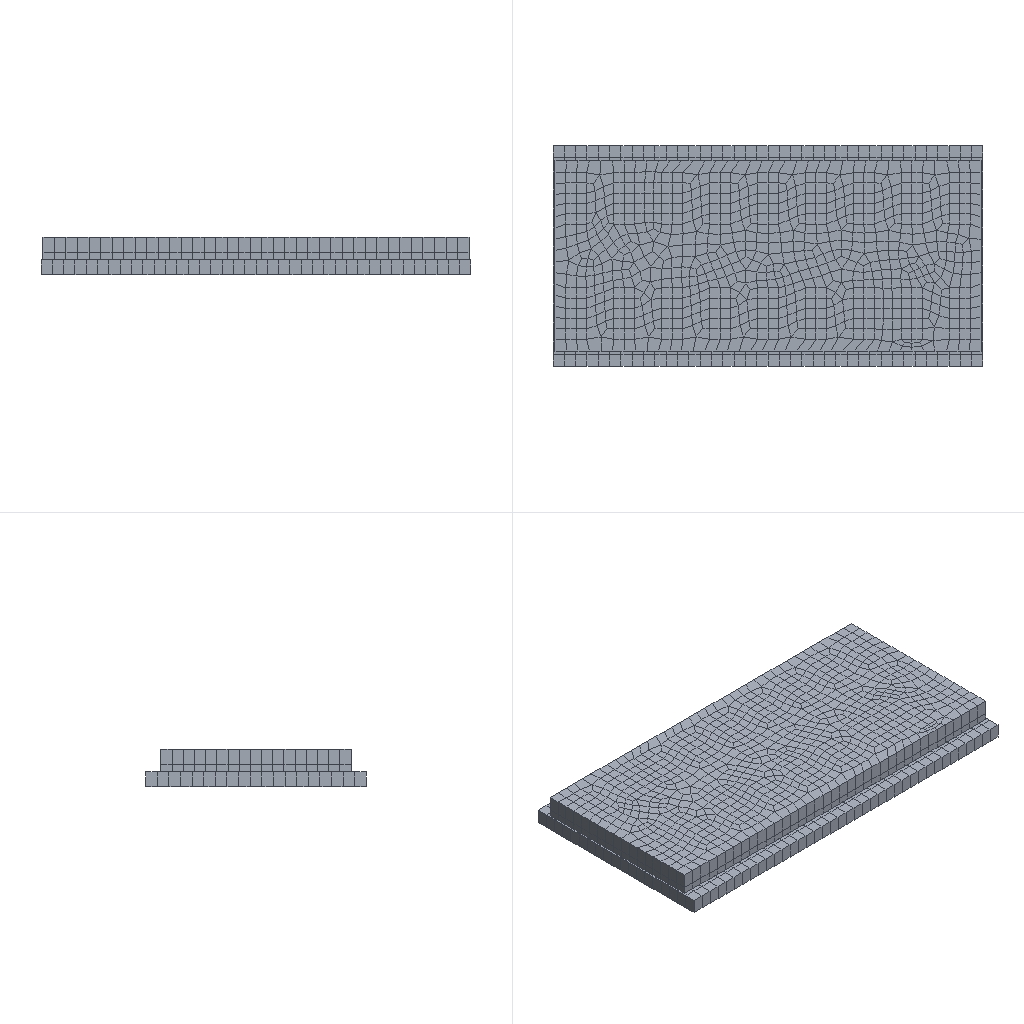Simulation study | abaqus
Set-up summary:
category,name,step,type,value,unit,region
solver,abaqus
solver,version,,,Abaqus/Standard 2020
units,not stated in the deck,,not stated
analysis,deck,,static,static
load_step,Step-1,Step-1,static
load_step,requested,,,1
mesh,nodes,,,5088
mesh,elements,,,2556
element_type,T3D2,,truss,400
element_type,C3D8R,,solid,2156
load,load commands in deck,,count,2
bc,support commands in deck,,count,1
material,DIZUOANDCHONGTIAN,,in results
material,GUIDAO,,in results
material,STEEL,,in results
check,setup vs results,,match,"per instance, exact: element labels, types and connectivity; labels of the nodes the elements use; coordinates of those nodes at SINGLE_PRECISION in 43 of 43 instance(s)"
Abaqus input file, long lists of numbers shortened:
*Heading
** Job name: Job-1 Model name: Model-1
** Generated by: Abaqus/CAE 2020
*Preprint, echo=NO, model=NO, history=NO, contact=NO
**
** PARTS
**
*Part, name=chongtian
*Node
      1,           0.,       -2500.,          94.
      2,           0.,  -2352.941,          94.
** (1366 more lines like these left out)
*Element, type=C3D8R
  1,   37,   38,   56,   55,    1,    2,   20,   19
  2,   38,   39,   57,   56,    2,    3,   21,   20
** (627 more lines like these left out)
*Nset, nset=Set-1, generate
    1,  1368,     1
*Elset, elset=Set-1, generate
   1,  629,    1
** Section: chongtian
*Solid Section, elset=Set-1, material=dizuoandchongtian
,
*End Part
**
*Part, name=dizuo
*Node
      1,           0.,       -2900.,         196.
      2,           0.,  -2747.368,         196.
** (1558 more lines like these left out)
*Element, type=C3D8R
  1,   41,   42,   62,   61,    1,    2,   22,   21
  2,   42,   43,   63,   62,    2,    3,   23,   22
** (720 more lines like these left out)
*Nset, nset=Set-1, generate
    1,  1560,     1
*Elset, elset=Set-1, generate
   1,  722,    1
** Section: chongtian
*Solid Section, elset=Set-1, material=dizuoandchongtian
,
*End Part
**
*Part, name=guidao
*Node
      1,       5182.5,       -1669.,         200.
      2,       5182.5,       -2344.,         200.
** (1718 more lines like these left out)
*Element, type=C3D8R
  1,   86,  361,   77,    1,  946, 1221,  937,  861
  2,  361,  362,   78,   77, 1221, 1222,  938,  937
** (803 more lines like these left out)
*Nset, nset=Set-1, generate
    1,  1720,     1
*Elset, elset=Set-1, generate
   1,  805,    1
** Section: guidao
*Solid Section, elset=Set-1, material=guidao
,
*End Part
**
*Part, name=heng-jin
*Node
      1,           0.,           0.,           0.
      2,           0.,       -243.5,           0.
** (9 more lines like these left out)
*Element, type=T3D2
 1,  1,  2
 2,  2,  3
** (8 more lines like these left out)
*Nset, nset=Set-2, generate
  1,  11,   1
*Elset, elset=Set-2, generate
  1,  10,   1
** Section: steel
*Solid Section, elset=Set-2, material=steel
78.5,
*End Part
**
*Part, name=zong-jin
*Node
      1,           0.,           0.,           0.
      2,           0.,        -552.,           0.
** (9 more lines like these left out)
*Element, type=T3D2
 1,  1,  2
 2,  2,  3
** (8 more lines like these left out)
*Nset, nset=Set-2, generate
  1,  11,   1
*Elset, elset=Set-2, generate
  1,  10,   1
** Section: steel
*Solid Section, elset=Set-2, material=steel
78.5,
*End Part
**
**
** ASSEMBLY
**
*Assembly, name=Assembly
**
*Instance, name=chongtian-1, part=chongtian
         25.,        -200.,         196.
*End Instance
**
*Instance, name=dizuo-1, part=dizuo
*End Instance
**
*Instance, name=guidao-1, part=guidao
         25.,        -200.,         290.
*End Instance
**
*Instance, name=heng-jin-1, part=heng-jin
        175.,       -232.5,         390.
*End Instance
**
*Instance, name=zong-jin-1, part=zong-jin
         75.,       -232.5,         350.
         75.,       -232.5,         350.,          75.,       -232.5, 351., 90.
*End Instance
**
*Instance, name=zong-jin-1-lin-1-2-1, part=zong-jin
         75.,       -572.5,         350.
         75.,       -572.5,         350.,          75.,       -572.5, 351., 90.
*End Instance
**
*Instance, name=zong-jin-1-lin-1-3, part=zong-jin
         75.,       -912.5,         350.
         75.,       -912.5,         350.,          75.,       -912.5, 351., 90.
*End Instance
**
*Instance, name=zong-jin-1-lin-1-4, part=zong-jin
         75.,      -1252.5,         350.
         75.,      -1252.5,         350.,          75.,      -1252.5, 351., 90.
*End Instance
**
*Instance, name=zong-jin-1-lin-1-5, part=zong-jin
         75.,      -1592.5,         350.
         75.,      -1592.5,         350.,          75.,      -1592.5, 351., 90.
*End Instance
**
*Instance, name=zong-jin-1-lin-1-6, part=zong-jin
         75.,      -1932.5,         350.
         75.,      -1932.5,         350.,          75.,      -1932.5, 351., 90.
*End Instance
**
*Instance, name=zong-jin-1-lin-1-7, part=zong-jin
         75.,      -2272.5,         350.
         75.,      -2272.5,         350.,          75.,      -2272.5, 351., 90.
*End Instance
**
*Instance, name=zong-jin-1-lin-1-8, part=zong-jin
         75.,      -2612.5,         350.
         75.,      -2612.5,         350.,          75.,      -2612.5, 351., 90.
*End Instance
**
*Instance, name=zong-jin-1-lin-2-1-1, part=zong-jin
         75.,       -232.5,         430.
         75.,       -232.5,         430.,          75.,       -232.5, 431., 90.
*End Instance
**
*Instance, name=zong-jin-1-lin-2-2-1, part=zong-jin
         75.,       -572.5,         430.
         75.,       -572.5,         430.,          75.,       -572.5, 431., 90.
*End Instance
**
*Instance, name=zong-jin-1-lin-2-3, part=zong-jin
         75.,       -912.5,         430.
         75.,       -912.5,         430.,          75.,       -912.5, 431., 90.
*End Instance
**
*Instance, name=zong-jin-1-lin-2-4, part=zong-jin
         75.,      -1252.5,         430.
         75.,      -1252.5,         430.,          75.,      -1252.5, 431., 90.
*End Instance
**
*Instance, name=zong-jin-1-lin-2-5, part=zong-jin
         75.,      -1592.5,         430.
         75.,      -1592.5,         430.,          75.,      -1592.5, 431., 90.
*End Instance
**
*Instance, name=zong-jin-1-lin-2-6, part=zong-jin
         75.,      -1932.5,         430.
         75.,      -1932.5,         430.,          75.,      -1932.5, 431., 90.
*End Instance
**
*Instance, name=zong-jin-1-lin-2-7, part=zong-jin
         75.,      -2272.5,         430.
         75.,      -2272.5,         430.,          75.,      -2272.5, 431., 90.
*End Instance
**
*Instance, name=zong-jin-1-lin-2-8, part=zong-jin
         75.,      -2612.5,         430.
         75.,      -2612.5,         430.,          75.,      -2612.5, 431., 90.
*End Instance
**
*Instance, name=heng-jin-1-lin-2-1-1, part=heng-jin
        405.,       -232.5,         390.
*End Instance
**
*Instance, name=heng-jin-1-lin-3-1-1, part=heng-jin
        635.,       -232.5,         390.
*End Instance
**
*Instance, name=heng-jin-1-lin-4-1-1, part=heng-jin
        865.,       -232.5,         390.
*End Instance
**
*Instance, name=heng-jin-1-lin-5-1-1, part=heng-jin
       1095.,       -232.5,         390.
*End Instance
**
*Instance, name=heng-jin-1-lin-6-1-1, part=heng-jin
       1325.,       -232.5,         390.
*End Instance
**
*Instance, name=heng-jin-1-lin-7-1-1, part=heng-jin
       1555.,       -232.5,         390.
*End Instance
**
*Instance, name=heng-jin-1-lin-8-1-1, part=heng-jin
       1785.,       -232.5,         390.
*End Instance
**
*Instance, name=heng-jin-1-lin-9-1, part=heng-jin
       2015.,       -232.5,         390.
*End Instance
**
*Instance, name=heng-jin-1-lin-10-1, part=heng-jin
       2245.,       -232.5,         390.
*End Instance
**
*Instance, name=heng-jin-1-lin-11-1, part=heng-jin
       2475.,       -232.5,         390.
*End Instance
**
*Instance, name=heng-jin-1-lin-12-1, part=heng-jin
       2705.,       -232.5,         390.
*End Instance
**
*Instance, name=heng-jin-1-lin-13-1, part=heng-jin
       2935.,       -232.5,         390.
*End Instance
**
*Instance, name=heng-jin-1-lin-14-1, part=heng-jin
       3165.,       -232.5,         390.
*End Instance
**
*Instance, name=heng-jin-1-lin-15-1, part=heng-jin
       3395.,       -232.5,         390.
*End Instance
**
*Instance, name=heng-jin-1-lin-16-1, part=heng-jin
       3625.,       -232.5,         390.
*End Instance
**
*Instance, name=heng-jin-1-lin-17-1, part=heng-jin
       3855.,       -232.5,         390.
*End Instance
**
*Instance, name=heng-jin-1-lin-18-1, part=heng-jin
       4085.,       -232.5,         390.
*End Instance
**
*Instance, name=heng-jin-1-lin-19-1, part=heng-jin
       4315.,       -232.5,         390.
*End Instance
**
*Instance, name=heng-jin-1-lin-20-1, part=heng-jin
       4545.,       -232.5,         390.
*End Instance
**
*Instance, name=heng-jin-1-lin-21-1, part=heng-jin
       4775.,       -232.5,         390.
*End Instance
**
*Instance, name=heng-jin-1-lin-22-1, part=heng-jin
       5005.,       -232.5,         390.
*End Instance
**
*Instance, name=heng-jin-1-lin-23-1, part=heng-jin
       5235.,       -232.5,         390.
*End Instance
**
*Instance, name=heng-jin-1-lin-24-1, part=heng-jin
       5465.,       -232.5,         390.
*End Instance
**
*Nset, nset=Set-3, instance=heng-jin-1, generate
  1,  11,   1
*Nset, nset=Set-3, instance=zong-jin-1, generate
  1,  11,   1
*Elset, elset=Set-3, instance=heng-jin-1, generate
  1,  10,   1
*Elset, elset=Set-3, instance=zong-jin-1, generate
  1,  10,   1
*Nset, nset=Set-4, instance=dizuo-1
   21,   22,   23,   24,   25,   26,   27,   28,   29,   30,   31,   32,   33,   34,   35,   36
   37,   38,   39,   40,   61,   62,   63,   64,   65,   66,   67,   68,   69,   70,   71,   72
** (47 more lines like these left out)
*Elset, elset=Set-4, instance=dizuo-1, generate
   1,  722,    1
*Nset, nset=Set-7, instance=heng-jin-1, generate
  1,  11,   1
*Nset, nset=Set-7, instance=zong-jin-1, generate
  1,  11,   1
*Nset, nset=Set-7, instance=zong-jin-1-lin-1-2-1, generate
  1,  11,   1
*Nset, nset=Set-7, instance=zong-jin-1-lin-1-4, generate
  1,  11,   1
*Nset, nset=Set-7, instance=zong-jin-1-lin-1-6, generate
  1,  11,   1
*Nset, nset=Set-7, instance=zong-jin-1-lin-2-6, generate
  1,  11,   1
*Nset, nset=Set-7, instance=heng-jin-1-lin-7-1-1, generate
  1,  11,   1
*Nset, nset=Set-7, instance=heng-jin-1-lin-23-1, generate
  1,  11,   1
*Nset, nset=Set-7, instance=heng-jin-1-lin-15-1, generate
  1,  11,   1
*Nset, nset=Set-7, instance=zong-jin-1-lin-2-2-1, generate
  1,  11,   1
*Nset, nset=Set-7, instance=heng-jin-1-lin-11-1, generate
  1,  11,   1
*Nset, nset=Set-7, instance=heng-jin-1-lin-3-1-1, generate
  1,  11,   1
*Nset, nset=Set-7, instance=heng-jin-1-lin-19-1, generate
  1,  11,   1
*Nset, nset=Set-7, instance=zong-jin-1-lin-1-8, generate
  1,  11,   1
*Nset, nset=Set-7, instance=zong-jin-1-lin-2-8, generate
  1,  11,   1
*Nset, nset=Set-7, instance=heng-jin-1-lin-9-1, generate
  1,  11,   1
*Nset, nset=Set-7, instance=heng-jin-1-lin-17-1, generate
  1,  11,   1
*Nset, nset=Set-7, instance=zong-jin-1-lin-2-4, generate
  1,  11,   1
*Nset, nset=Set-7, instance=heng-jin-1-lin-13-1, generate
  1,  11,   1
*Nset, nset=Set-7, instance=heng-jin-1-lin-5-1-1, generate
  1,  11,   1
*Nset, nset=Set-7, instance=heng-jin-1-lin-21-1, generate
  1,  11,   1
*Nset, nset=Set-7, instance=zong-jin-1-lin-1-3, generate
  1,  11,   1
*Nset, nset=Set-7, instance=zong-jin-1-lin-1-7, generate
  1,  11,   1
*Nset, nset=Set-7, instance=zong-jin-1-lin-2-7, generate
  1,  11,   1
*Nset, nset=Set-7, instance=heng-jin-1-lin-8-1-1, generate
  1,  11,   1
*Nset, nset=Set-7, instance=heng-jin-1-lin-24-1, generate
  1,  11,   1
*Nset, nset=Set-7, instance=heng-jin-1-lin-16-1, generate
  1,  11,   1
*Nset, nset=Set-7, instance=zong-jin-1-lin-2-3, generate
  1,  11,   1
*Nset, nset=Set-7, instance=heng-jin-1-lin-12-1, generate
  1,  11,   1
*Nset, nset=Set-7, instance=heng-jin-1-lin-4-1-1, generate
  1,  11,   1
*Nset, nset=Set-7, instance=heng-jin-1-lin-20-1, generate
  1,  11,   1
*Nset, nset=Set-7, instance=zong-jin-1-lin-1-5, generate
  1,  11,   1
*Nset, nset=Set-7, instance=zong-jin-1-lin-2-1-1, generate
  1,  11,   1
*Nset, nset=Set-7, instance=heng-jin-1-lin-10-1, generate
  1,  11,   1
*Nset, nset=Set-7, instance=heng-jin-1-lin-2-1-1, generate
  1,  11,   1
*Nset, nset=Set-7, instance=heng-jin-1-lin-18-1, generate
  1,  11,   1
*Nset, nset=Set-7, instance=zong-jin-1-lin-2-5, generate
  1,  11,   1
*Nset, nset=Set-7, instance=heng-jin-1-lin-14-1, generate
  1,  11,   1
*Nset, nset=Set-7, instance=heng-jin-1-lin-6-1-1, generate
  1,  11,   1
*Nset, nset=Set-7, instance=heng-jin-1-lin-22-1, generate
  1,  11,   1
*Elset, elset=Set-7, instance=heng-jin-1, generate
  1,  10,   1
*Elset, elset=Set-7, instance=zong-jin-1, generate
  1,  10,   1
*Elset, elset=Set-7, instance=zong-jin-1-lin-1-2-1, generate
  1,  10,   1
*Elset, elset=Set-7, instance=zong-jin-1-lin-1-4, generate
  1,  10,   1
*Elset, elset=Set-7, instance=zong-jin-1-lin-1-6, generate
  1,  10,   1
*Elset, elset=Set-7, instance=zong-jin-1-lin-2-6, generate
  1,  10,   1
*Elset, elset=Set-7, instance=heng-jin-1-lin-7-1-1, generate
  1,  10,   1
*Elset, elset=Set-7, instance=heng-jin-1-lin-23-1, generate
  1,  10,   1
*Elset, elset=Set-7, instance=heng-jin-1-lin-15-1, generate
  1,  10,   1
*Elset, elset=Set-7, instance=zong-jin-1-lin-2-2-1, generate
  1,  10,   1
*Elset, elset=Set-7, instance=heng-jin-1-lin-11-1, generate
  1,  10,   1
*Elset, elset=Set-7, instance=heng-jin-1-lin-3-1-1, generate
  1,  10,   1
*Elset, elset=Set-7, instance=heng-jin-1-lin-19-1, generate
  1,  10,   1
*Elset, elset=Set-7, instance=zong-jin-1-lin-1-8, generate
  1,  10,   1
*Elset, elset=Set-7, instance=zong-jin-1-lin-2-8, generate
  1,  10,   1
*Elset, elset=Set-7, instance=heng-jin-1-lin-9-1, generate
  1,  10,   1
*Elset, elset=Set-7, instance=heng-jin-1-lin-17-1, generate
  1,  10,   1
*Elset, elset=Set-7, instance=zong-jin-1-lin-2-4, generate
  1,  10,   1
*Elset, elset=Set-7, instance=heng-jin-1-lin-13-1, generate
  1,  10,   1
*Elset, elset=Set-7, instance=heng-jin-1-lin-5-1-1, generate
  1,  10,   1
*Elset, elset=Set-7, instance=heng-jin-1-lin-21-1, generate
  1,  10,   1
*Elset, elset=Set-7, instance=zong-jin-1-lin-1-3, generate
  1,  10,   1
*Elset, elset=Set-7, instance=zong-jin-1-lin-1-7, generate
  1,  10,   1
*Elset, elset=Set-7, instance=zong-jin-1-lin-2-7, generate
  1,  10,   1
*Elset, elset=Set-7, instance=heng-jin-1-lin-8-1-1, generate
  1,  10,   1
*Elset, elset=Set-7, instance=heng-jin-1-lin-24-1, generate
  1,  10,   1
*Elset, elset=Set-7, instance=heng-jin-1-lin-16-1, generate
  1,  10,   1
*Elset, elset=Set-7, instance=zong-jin-1-lin-2-3, generate
  1,  10,   1
*Elset, elset=Set-7, instance=heng-jin-1-lin-12-1, generate
  1,  10,   1
*Elset, elset=Set-7, instance=heng-jin-1-lin-4-1-1, generate
  1,  10,   1
*Elset, elset=Set-7, instance=heng-jin-1-lin-20-1, generate
  1,  10,   1
*Elset, elset=Set-7, instance=zong-jin-1-lin-1-5, generate
  1,  10,   1
*Elset, elset=Set-7, instance=zong-jin-1-lin-2-1-1, generate
  1,  10,   1
*Elset, elset=Set-7, instance=heng-jin-1-lin-10-1, generate
  1,  10,   1
*Elset, elset=Set-7, instance=heng-jin-1-lin-2-1-1, generate
  1,  10,   1
*Elset, elset=Set-7, instance=heng-jin-1-lin-18-1, generate
  1,  10,   1
*Elset, elset=Set-7, instance=zong-jin-1-lin-2-5, generate
  1,  10,   1
*Elset, elset=Set-7, instance=heng-jin-1-lin-14-1, generate
  1,  10,   1
*Elset, elset=Set-7, instance=heng-jin-1-lin-6-1-1, generate
  1,  10,   1
*Elset, elset=Set-7, instance=heng-jin-1-lin-22-1, generate
  1,  10,   1
*Nset, nset=m_Set-1, instance=heng-jin-1, generate
  1,  11,   1
*Nset, nset=m_Set-1, instance=zong-jin-1, generate
  1,  11,   1
*Elset, elset=m_Set-1, instance=heng-jin-1, generate
  1,  10,   1
*Elset, elset=m_Set-1, instance=zong-jin-1, generate
  1,  10,   1
*Nset, nset=m_Set-5, instance=heng-jin-1, generate
  1,  11,   1
*Nset, nset=m_Set-5, instance=zong-jin-1, generate
  1,  11,   1
*Nset, nset=m_Set-5, instance=zong-jin-1-lin-1-2-1, generate
  1,  11,   1
*Nset, nset=m_Set-5, instance=zong-jin-1-lin-1-4, generate
  1,  11,   1
*Nset, nset=m_Set-5, instance=zong-jin-1-lin-1-6, generate
  1,  11,   1
*Nset, nset=m_Set-5, instance=zong-jin-1-lin-2-6, generate
  1,  11,   1
*Nset, nset=m_Set-5, instance=heng-jin-1-lin-7-1-1, generate
  1,  11,   1
*Nset, nset=m_Set-5, instance=heng-jin-1-lin-23-1, generate
  1,  11,   1
*Nset, nset=m_Set-5, instance=heng-jin-1-lin-15-1, generate
  1,  11,   1
*Nset, nset=m_Set-5, instance=zong-jin-1-lin-2-2-1, generate
  1,  11,   1
*Nset, nset=m_Set-5, instance=heng-jin-1-lin-11-1, generate
  1,  11,   1
*Nset, nset=m_Set-5, instance=heng-jin-1-lin-3-1-1, generate
  1,  11,   1
*Nset, nset=m_Set-5, instance=heng-jin-1-lin-19-1, generate
  1,  11,   1
*Nset, nset=m_Set-5, instance=zong-jin-1-lin-1-8, generate
  1,  11,   1
*Nset, nset=m_Set-5, instance=zong-jin-1-lin-2-8, generate
  1,  11,   1
*Nset, nset=m_Set-5, instance=heng-jin-1-lin-9-1, generate
  1,  11,   1
*Nset, nset=m_Set-5, instance=heng-jin-1-lin-17-1, generate
  1,  11,   1
*Nset, nset=m_Set-5, instance=zong-jin-1-lin-2-4, generate
  1,  11,   1
*Nset, nset=m_Set-5, instance=heng-jin-1-lin-13-1, generate
  1,  11,   1
*Nset, nset=m_Set-5, instance=heng-jin-1-lin-5-1-1, generate
  1,  11,   1
*Nset, nset=m_Set-5, instance=heng-jin-1-lin-21-1, generate
  1,  11,   1
*Nset, nset=m_Set-5, instance=zong-jin-1-lin-1-3, generate
  1,  11,   1
*Nset, nset=m_Set-5, instance=zong-jin-1-lin-1-7, generate
  1,  11,   1
*Nset, nset=m_Set-5, instance=zong-jin-1-lin-2-7, generate
  1,  11,   1
*Nset, nset=m_Set-5, instance=heng-jin-1-lin-8-1-1, generate
  1,  11,   1
*Nset, nset=m_Set-5, instance=heng-jin-1-lin-24-1, generate
  1,  11,   1
*Nset, nset=m_Set-5, instance=heng-jin-1-lin-16-1, generate
  1,  11,   1
*Nset, nset=m_Set-5, instance=zong-jin-1-lin-2-3, generate
  1,  11,   1
*Nset, nset=m_Set-5, instance=heng-jin-1-lin-12-1, generate
  1,  11,   1
*Nset, nset=m_Set-5, instance=heng-jin-1-lin-4-1-1, generate
  1,  11,   1
*Nset, nset=m_Set-5, instance=heng-jin-1-lin-20-1, generate
  1,  11,   1
*Nset, nset=m_Set-5, instance=zong-jin-1-lin-1-5, generate
  1,  11,   1
*Nset, nset=m_Set-5, instance=zong-jin-1-lin-2-1-1, generate
  1,  11,   1
*Nset, nset=m_Set-5, instance=heng-jin-1-lin-10-1, generate
  1,  11,   1
*Nset, nset=m_Set-5, instance=heng-jin-1-lin-2-1-1, generate
  1,  11,   1
*Nset, nset=m_Set-5, instance=heng-jin-1-lin-18-1, generate
  1,  11,   1
*Nset, nset=m_Set-5, instance=zong-jin-1-lin-2-5, generate
  1,  11,   1
*Nset, nset=m_Set-5, instance=heng-jin-1-lin-14-1, generate
  1,  11,   1
*Nset, nset=m_Set-5, instance=heng-jin-1-lin-6-1-1, generate
  1,  11,   1
*Nset, nset=m_Set-5, instance=heng-jin-1-lin-22-1, generate
  1,  11,   1
*Elset, elset=m_Set-5, instance=heng-jin-1, generate
  1,  10,   1
*Elset, elset=m_Set-5, instance=zong-jin-1, generate
  1,  10,   1
*Elset, elset=m_Set-5, instance=zong-jin-1-lin-1-2-1, generate
  1,  10,   1
*Elset, elset=m_Set-5, instance=zong-jin-1-lin-1-4, generate
  1,  10,   1
*Elset, elset=m_Set-5, instance=zong-jin-1-lin-1-6, generate
  1,  10,   1
*Elset, elset=m_Set-5, instance=zong-jin-1-lin-2-6, generate
  1,  10,   1
*Elset, elset=m_Set-5, instance=heng-jin-1-lin-7-1-1, generate
  1,  10,   1
*Elset, elset=m_Set-5, instance=heng-jin-1-lin-23-1, generate
  1,  10,   1
*Elset, elset=m_Set-5, instance=heng-jin-1-lin-15-1, generate
  1,  10,   1
*Elset, elset=m_Set-5, instance=zong-jin-1-lin-2-2-1, generate
  1,  10,   1
*Elset, elset=m_Set-5, instance=heng-jin-1-lin-11-1, generate
  1,  10,   1
*Elset, elset=m_Set-5, instance=heng-jin-1-lin-3-1-1, generate
  1,  10,   1
*Elset, elset=m_Set-5, instance=heng-jin-1-lin-19-1, generate
  1,  10,   1
*Elset, elset=m_Set-5, instance=zong-jin-1-lin-1-8, generate
  1,  10,   1
*Elset, elset=m_Set-5, instance=zong-jin-1-lin-2-8, generate
  1,  10,   1
*Elset, elset=m_Set-5, instance=heng-jin-1-lin-9-1, generate
  1,  10,   1
*Elset, elset=m_Set-5, instance=heng-jin-1-lin-17-1, generate
  1,  10,   1
*Elset, elset=m_Set-5, instance=zong-jin-1-lin-2-4, generate
  1,  10,   1
*Elset, elset=m_Set-5, instance=heng-jin-1-lin-13-1, generate
  1,  10,   1
*Elset, elset=m_Set-5, instance=heng-jin-1-lin-5-1-1, generate
  1,  10,   1
*Elset, elset=m_Set-5, instance=heng-jin-1-lin-21-1, generate
  1,  10,   1
*Elset, elset=m_Set-5, instance=zong-jin-1-lin-1-3, generate
  1,  10,   1
*Elset, elset=m_Set-5, instance=zong-jin-1-lin-1-7, generate
  1,  10,   1
*Elset, elset=m_Set-5, instance=zong-jin-1-lin-2-7, generate
  1,  10,   1
*Elset, elset=m_Set-5, instance=heng-jin-1-lin-8-1-1, generate
  1,  10,   1
*Elset, elset=m_Set-5, instance=heng-jin-1-lin-24-1, generate
  1,  10,   1
*Elset, elset=m_Set-5, instance=heng-jin-1-lin-16-1, generate
  1,  10,   1
*Elset, elset=m_Set-5, instance=zong-jin-1-lin-2-3, generate
  1,  10,   1
*Elset, elset=m_Set-5, instance=heng-jin-1-lin-12-1, generate
  1,  10,   1
*Elset, elset=m_Set-5, instance=heng-jin-1-lin-4-1-1, generate
  1,  10,   1
*Elset, elset=m_Set-5, instance=heng-jin-1-lin-20-1, generate
  1,  10,   1
*Elset, elset=m_Set-5, instance=zong-jin-1-lin-1-5, generate
  1,  10,   1
*Elset, elset=m_Set-5, instance=zong-jin-1-lin-2-1-1, generate
  1,  10,   1
*Elset, elset=m_Set-5, instance=heng-jin-1-lin-10-1, generate
  1,  10,   1
*Elset, elset=m_Set-5, instance=heng-jin-1-lin-2-1-1, generate
  1,  10,   1
*Elset, elset=m_Set-5, instance=heng-jin-1-lin-18-1, generate
  1,  10,   1
*Elset, elset=m_Set-5, instance=zong-jin-1-lin-2-5, generate
  1,  10,   1
*Elset, elset=m_Set-5, instance=heng-jin-1-lin-14-1, generate
  1,  10,   1
*Elset, elset=m_Set-5, instance=heng-jin-1-lin-6-1-1, generate
  1,  10,   1
*Elset, elset=m_Set-5, instance=heng-jin-1-lin-22-1, generate
  1,  10,   1
*Nset, nset=s_Set-1, instance=guidao-1, generate
    1,  1720,     1
*Elset, elset=s_Set-1, instance=guidao-1, generate
   1,  805,    1
*Nset, nset=s_Set-5, instance=guidao-1, generate
    1,  1720,     1
*Elset, elset=s_Set-5, instance=guidao-1, generate
   1,  805,    1
*Elset, elset=_Surf-1_S1, internal, instance=guidao-1, generate
   1,  180,    1
*Surface, type=ELEMENT, name=Surf-1
_Surf-1_S1, S1
*Elset, elset=_Surf-6_S1, internal, instance=guidao-1, generate
  51,  140,    1
*Surface, type=ELEMENT, name=Surf-6
_Surf-6_S1, S1
*Elset, elset=_m_Surf-2_S2, internal, instance=guidao-1, generate
   1,  805,    1
*Surface, type=ELEMENT, name=m_Surf-2
_m_Surf-2_S2, S2
*Elset, elset=_m_Surf-4_S5, internal, instance=chongtian-1, generate
   1,  629,    1
*Surface, type=ELEMENT, name=m_Surf-4
_m_Surf-4_S5, S5
*Elset, elset=_s_Surf-2_S3, internal, instance=chongtian-1, generate
   1,  629,    1
*Surface, type=ELEMENT, name=s_Surf-2
_s_Surf-2_S3, S3
*Elset, elset=_s_Surf-4_S3, internal, instance=dizuo-1, generate
   1,  722,    1
*Surface, type=ELEMENT, name=s_Surf-4
_s_Surf-4_S3, S3
** Constraint: Constraint-1
*Embedded Element, host elset=s_Set-5
m_Set-5
*End Assembly
*Amplitude, name=Amp-1
             0.,              0.,              1.,              1.
**
** MATERIALS
**
*Material, name=dizuoandchongtian
*Density
 2.4e-09,
*Elastic
32500., 0.2
*Expansion
 1.1e-05,
*Material, name=guidao
*Density
 2.5e-09,
*Elastic
36000., 0.2
*Expansion
 1e-05,
*Material, name=steel
*Density
 7.8e-09,
*Elastic
210000., 0.3
*Plastic
400.,0.
**
** INTERACTION PROPERTIES
**
*Surface Interaction, name=IntProp-1
1.,
*Friction, slip tolerance=0.005
 0.8,
*Surface Behavior, pressure-overclosure=HARD
**
** PREDEFINED FIELDS
**
** Name: Predefined Field-1   Type: Stress
*Initial Conditions, type=STRESS
Set-7, -1., -1., -1.,
**
** INTERACTIONS
**
** Interaction: Int-1
*Contact Pair, interaction=IntProp-1, type=SURFACE TO SURFACE
s_Surf-2, m_Surf-2
** Interaction: Int-2
*Contact Pair, interaction=IntProp-1, type=SURFACE TO SURFACE
s_Surf-4, m_Surf-4
** ----------------------------------------------------------------
**
** STEP: Step-1
**
*Step, name=Step-1, nlgeom=YES, inc=1000
*Static, stabilize=0.0002, allsdtol=0.05, continue=NO
0.01, 1., 1e-05, 1.
**
** BOUNDARY CONDITIONS
**
** Name: BC-1 Type: 对称/反对称/完全固定
*Boundary
Set-4, ENCASTRE
**
** LOADS
**
** Name: Load-1   Type: Pressure
*Dsload, amplitude=Amp-1
Surf-1, P, 3.2
** Name: Load-2   Type: Surface traction
*Dsload, amplitude=Amp-1
Surf-6, TRVEC, 1., 0., -1., 0.
**
** OUTPUT REQUESTS
**
*Restart, write, frequency=0
**
** FIELD OUTPUT: F-Output-1
**
*Output, field
*Node Output
CF, RF, U, V
*Element Output, directions=YES
E, LE, MISES, PE, PEEQ, PEMAG, S, SSAVG
*Contact Output
CDISP, CSTRESS
**
** HISTORY OUTPUT: H-Output-1
**
*Output, history, variable=PRESELECT
*End Step
Results summary:
result,step,,completed,increments=11 time=1.0/1.0
result,analysis,,,static
result,last_loadstep,,,1
result,primary field,,,U
result,reaction total,,FX,14.306,model units
result,reaction total,,FY,1669258.847,model units
result,reaction total,,FZ,10686498.885,model units